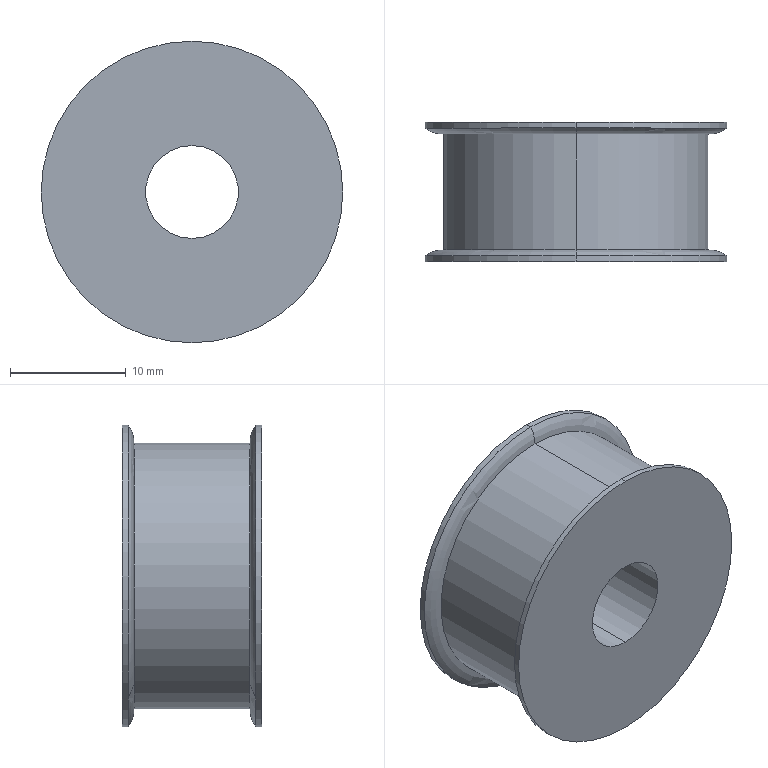Part | SolidWorks | features Revolution 2 | 1 solid | 14 faces | box 26 x 12 x 26 mm | volume 4546 mm3 | cylinder 8 | torus 4 | plane 2 | commonest cylinder face diameters 26 x4 8 x2 22.92 x2
STEP:
#1=CARTESIAN_POINT('',(0.,-5.5,-13.));
#2=VERTEX_POINT('',#1);
#3=CARTESIAN_POINT('',(0.,-5.5,13.));
#4=VERTEX_POINT('',#3);
#5=CARTESIAN_POINT('',(0.,-5.5,0.));
#6=DIRECTION('',(0.,-1.,0.));
#7=DIRECTION('',(0.,0.,-1.));
#8=AXIS2_PLACEMENT_3D('',#5,#6,#7);
#9=CIRCLE('',#8,13.);
#10=EDGE_CURVE('',#2,#4,#9,.T.);
#11=ORIENTED_EDGE('',*,*,#10,.T.);
#12=CARTESIAN_POINT('',(0.,-6.,13.));
#13=VERTEX_POINT('',#12);
#14=CARTESIAN_POINT('',(0.,0.,13.));
#15=DIRECTION('',(0.,-1.,0.));
#16=VECTOR('',#15,1000.);
#17=LINE('',#14,#16);
#18=EDGE_CURVE('',#4,#13,#17,.T.);
#19=ORIENTED_EDGE('',*,*,#18,.T.);
#20=CARTESIAN_POINT('',(0.,-6.,-13.));
#21=VERTEX_POINT('',#20);
#22=CARTESIAN_POINT('',(0.,-6.,0.));
#23=DIRECTION('',(0.,-1.,0.));
#24=DIRECTION('',(0.,0.,-1.));
#25=AXIS2_PLACEMENT_3D('',#22,#23,#24);
#26=CIRCLE('',#25,13.);
#27=EDGE_CURVE('',#21,#13,#26,.T.);
#28=ORIENTED_EDGE('',*,*,#27,.F.);
#29=CARTESIAN_POINT('',(0.,0.,-13.));
#30=DIRECTION('',(0.,-1.,0.));
#31=VECTOR('',#30,1000.);
#32=LINE('',#29,#31);
#33=EDGE_CURVE('',#2,#21,#32,.T.);
#34=ORIENTED_EDGE('',*,*,#33,.F.);
#35=EDGE_LOOP('',(#11,#19,#28,#34));
#36=FACE_OUTER_BOUND('',#35,.T.);
#37=CARTESIAN_POINT('',(0.,0.,0.));
#38=DIRECTION('',(0.,-1.,0.));
#39=DIRECTION('',(0.,0.,-1.));
#40=AXIS2_PLACEMENT_3D('',#37,#38,#39);
#41=CYLINDRICAL_SURFACE('',#40,13.);
#42=ADVANCED_FACE('',(#36),#41,.T.);
#43=CARTESIAN_POINT('',(0.,-5.,-11.46));
#44=VERTEX_POINT('',#43);
#45=CARTESIAN_POINT('',(0.,-5.,11.46));
#46=VERTEX_POINT('',#45);
#47=CARTESIAN_POINT('',(0.,-5.,0.));
#48=DIRECTION('',(0.,-1.,0.));
#49=DIRECTION('',(0.,0.,-1.));
#50=AXIS2_PLACEMENT_3D('',#47,#48,#49);
#51=CIRCLE('',#50,11.46);
#52=EDGE_CURVE('',#44,#46,#51,.T.);
#53=ORIENTED_EDGE('',*,*,#52,.T.);
#54=CARTESIAN_POINT('',(0.,-7.622,11.46));
#55=DIRECTION('',(1.,0.,0.));
#56=DIRECTION('',(0.,0.,-1.));
#57=AXIS2_PLACEMENT_3D('',#54,#55,#56);
#58=CIRCLE('',#57,2.622);
#59=EDGE_CURVE('',#46,#4,#58,.T.);
#60=ORIENTED_EDGE('',*,*,#59,.T.);
#61=ORIENTED_EDGE('',*,*,#10,.F.);
#62=CARTESIAN_POINT('',(0.,-7.622,-11.46));
#63=DIRECTION('',(-1.,0.,0.));
#64=DIRECTION('',(0.,0.,1.));
#65=AXIS2_PLACEMENT_3D('',#62,#63,#64);
#66=CIRCLE('',#65,2.622);
#67=EDGE_CURVE('',#44,#2,#66,.T.);
#68=ORIENTED_EDGE('',*,*,#67,.F.);
#69=EDGE_LOOP('',(#53,#60,#61,#68));
#70=FACE_OUTER_BOUND('',#69,.T.);
#71=CARTESIAN_POINT('',(0.,-7.622,0.));
#72=DIRECTION('',(0.,-1.,0.));
#73=DIRECTION('',(0.,0.,-1.));
#74=AXIS2_PLACEMENT_3D('',#71,#72,#73);
#75=TOROIDAL_SURFACE('',#74,11.46,2.622);
#76=ADVANCED_FACE('',(#70),#75,.T.);
#77=CARTESIAN_POINT('',(0.,6.,-13.));
#78=VERTEX_POINT('',#77);
#79=CARTESIAN_POINT('',(0.,6.,13.));
#80=VERTEX_POINT('',#79);
#81=CARTESIAN_POINT('',(0.,6.,0.));
#82=DIRECTION('',(0.,-1.,0.));
#83=DIRECTION('',(0.,0.,-1.));
#84=AXIS2_PLACEMENT_3D('',#81,#82,#83);
#85=CIRCLE('',#84,13.);
#86=EDGE_CURVE('',#78,#80,#85,.T.);
#87=ORIENTED_EDGE('',*,*,#86,.T.);
#88=CARTESIAN_POINT('',(0.,5.5,13.));
#89=VERTEX_POINT('',#88);
#90=CARTESIAN_POINT('',(0.,0.,13.));
#91=DIRECTION('',(0.,-1.,0.));
#92=VECTOR('',#91,1000.);
#93=LINE('',#90,#92);
#94=EDGE_CURVE('',#80,#89,#93,.T.);
#95=ORIENTED_EDGE('',*,*,#94,.T.);
#96=CARTESIAN_POINT('',(0.,5.5,-13.));
#97=VERTEX_POINT('',#96);
#98=CARTESIAN_POINT('',(0.,5.5,0.));
#99=DIRECTION('',(0.,-1.,0.));
#100=DIRECTION('',(0.,0.,-1.));
#101=AXIS2_PLACEMENT_3D('',#98,#99,#100);
#102=CIRCLE('',#101,13.);
#103=EDGE_CURVE('',#97,#89,#102,.T.);
#104=ORIENTED_EDGE('',*,*,#103,.F.);
#105=CARTESIAN_POINT('',(0.,0.,-13.));
#106=DIRECTION('',(0.,-1.,0.));
#107=VECTOR('',#106,1000.);
#108=LINE('',#105,#107);
#109=EDGE_CURVE('',#78,#97,#108,.T.);
#110=ORIENTED_EDGE('',*,*,#109,.F.);
#111=EDGE_LOOP('',(#87,#95,#104,#110));
#112=FACE_OUTER_BOUND('',#111,.T.);
#113=CARTESIAN_POINT('',(0.,0.,0.));
#114=DIRECTION('',(0.,-1.,0.));
#115=DIRECTION('',(0.,0.,-1.));
#116=AXIS2_PLACEMENT_3D('',#113,#114,#115);
#117=CYLINDRICAL_SURFACE('',#116,13.);
#118=ADVANCED_FACE('',(#112),#117,.T.);
#119=ORIENTED_EDGE('',*,*,#103,.T.);
#120=CARTESIAN_POINT('',(0.,5.,11.46));
#121=VERTEX_POINT('',#120);
#122=CARTESIAN_POINT('',(0.,7.622,11.46));
#123=DIRECTION('',(1.,0.,0.));
#124=DIRECTION('',(0.,0.,-1.));
#125=AXIS2_PLACEMENT_3D('',#122,#123,#124);
#126=CIRCLE('',#125,2.622);
#127=EDGE_CURVE('',#89,#121,#126,.T.);
#128=ORIENTED_EDGE('',*,*,#127,.T.);
#129=CARTESIAN_POINT('',(0.,5.,-11.46));
#130=VERTEX_POINT('',#129);
#131=CARTESIAN_POINT('',(0.,5.,0.));
#132=DIRECTION('',(0.,-1.,0.));
#133=DIRECTION('',(0.,0.,-1.));
#134=AXIS2_PLACEMENT_3D('',#131,#132,#133);
#135=CIRCLE('',#134,11.46);
#136=EDGE_CURVE('',#130,#121,#135,.T.);
#137=ORIENTED_EDGE('',*,*,#136,.F.);
#138=CARTESIAN_POINT('',(0.,7.622,-11.46));
#139=DIRECTION('',(-1.,0.,0.));
#140=DIRECTION('',(0.,0.,1.));
#141=AXIS2_PLACEMENT_3D('',#138,#139,#140);
#142=CIRCLE('',#141,2.622);
#143=EDGE_CURVE('',#97,#130,#142,.T.);
#144=ORIENTED_EDGE('',*,*,#143,.F.);
#145=EDGE_LOOP('',(#119,#128,#137,#144));
#146=FACE_OUTER_BOUND('',#145,.T.);
#147=CARTESIAN_POINT('',(0.,7.622,0.));
#148=DIRECTION('',(0.,-1.,0.));
#149=DIRECTION('',(0.,0.,-1.));
#150=AXIS2_PLACEMENT_3D('',#147,#148,#149);
#151=TOROIDAL_SURFACE('',#150,11.46,2.622);
#152=ADVANCED_FACE('',(#146),#151,.T.);
#153=CARTESIAN_POINT('',(0.,6.,4.));
#154=VERTEX_POINT('',#153);
#155=CARTESIAN_POINT('',(0.,6.,-4.));
#156=VERTEX_POINT('',#155);
#157=CARTESIAN_POINT('',(0.,6.,0.));
#158=DIRECTION('',(0.,-1.,0.));
#159=DIRECTION('',(0.,0.,-1.));
#160=AXIS2_PLACEMENT_3D('',#157,#158,#159);
#161=CIRCLE('',#160,4.);
#162=EDGE_CURVE('',#154,#156,#161,.T.);
#163=ORIENTED_EDGE('',*,*,#162,.F.);
#164=CARTESIAN_POINT('',(0.,-6.,4.));
#165=VERTEX_POINT('',#164);
#166=CARTESIAN_POINT('',(0.,0.,4.));
#167=DIRECTION('',(0.,-1.,0.));
#168=VECTOR('',#167,1000.);
#169=LINE('',#166,#168);
#170=EDGE_CURVE('',#154,#165,#169,.T.);
#171=ORIENTED_EDGE('',*,*,#170,.T.);
#172=CARTESIAN_POINT('',(0.,-6.,-4.));
#173=VERTEX_POINT('',#172);
#174=CARTESIAN_POINT('',(0.,-6.,0.));
#175=DIRECTION('',(0.,-1.,0.));
#176=DIRECTION('',(0.,0.,-1.));
#177=AXIS2_PLACEMENT_3D('',#174,#175,#176);
#178=CIRCLE('',#177,4.);
#179=EDGE_CURVE('',#165,#173,#178,.T.);
#180=ORIENTED_EDGE('',*,*,#179,.T.);
#181=CARTESIAN_POINT('',(0.,0.,-4.));
#182=DIRECTION('',(0.,-1.,0.));
#183=VECTOR('',#182,1000.);
#184=LINE('',#181,#183);
#185=EDGE_CURVE('',#156,#173,#184,.T.);
#186=ORIENTED_EDGE('',*,*,#185,.F.);
#187=EDGE_LOOP('',(#163,#171,#180,#186));
#188=FACE_OUTER_BOUND('',#187,.T.);
#189=CARTESIAN_POINT('',(0.,0.,0.));
#190=DIRECTION('',(0.,-1.,0.));
#191=DIRECTION('',(0.,0.,-1.));
#192=AXIS2_PLACEMENT_3D('',#189,#190,#191);
#193=CYLINDRICAL_SURFACE('',#192,4.);
#194=ADVANCED_FACE('',(#188),#193,.F.);
#195=ORIENTED_EDGE('',*,*,#136,.T.);
#196=CARTESIAN_POINT('',(0.,0.,11.46));
#197=DIRECTION('',(0.,-1.,0.));
#198=VECTOR('',#197,1000.);
#199=LINE('',#196,#198);
#200=EDGE_CURVE('',#121,#46,#199,.T.);
#201=ORIENTED_EDGE('',*,*,#200,.T.);
#202=ORIENTED_EDGE('',*,*,#52,.F.);
#203=CARTESIAN_POINT('',(0.,0.,-11.46));
#204=DIRECTION('',(0.,-1.,0.));
#205=VECTOR('',#204,1000.);
#206=LINE('',#203,#205);
#207=EDGE_CURVE('',#130,#44,#206,.T.);
#208=ORIENTED_EDGE('',*,*,#207,.F.);
#209=EDGE_LOOP('',(#195,#201,#202,#208));
#210=FACE_OUTER_BOUND('',#209,.T.);
#211=CARTESIAN_POINT('',(0.,0.,0.));
#212=DIRECTION('',(0.,-1.,0.));
#213=DIRECTION('',(0.,0.,-1.));
#214=AXIS2_PLACEMENT_3D('',#211,#212,#213);
#215=CYLINDRICAL_SURFACE('',#214,11.46);
#216=ADVANCED_FACE('',(#210),#215,.T.);
#217=ORIENTED_EDGE('',*,*,#200,.F.);
#218=CARTESIAN_POINT('',(0.,5.,0.));
#219=DIRECTION('',(0.,-1.,0.));
#220=DIRECTION('',(0.,0.,-1.));
#221=AXIS2_PLACEMENT_3D('',#218,#219,#220);
#222=CIRCLE('',#221,11.46);
#223=EDGE_CURVE('',#121,#130,#222,.T.);
#224=ORIENTED_EDGE('',*,*,#223,.T.);
#225=ORIENTED_EDGE('',*,*,#207,.T.);
#226=CARTESIAN_POINT('',(0.,-5.,0.));
#227=DIRECTION('',(0.,-1.,0.));
#228=DIRECTION('',(0.,0.,-1.));
#229=AXIS2_PLACEMENT_3D('',#226,#227,#228);
#230=CIRCLE('',#229,11.46);
#231=EDGE_CURVE('',#46,#44,#230,.T.);
#232=ORIENTED_EDGE('',*,*,#231,.F.);
#233=EDGE_LOOP('',(#217,#224,#225,#232));
#234=FACE_OUTER_BOUND('',#233,.T.);
#235=CARTESIAN_POINT('',(0.,0.,0.));
#236=DIRECTION('',(0.,-1.,0.));
#237=DIRECTION('',(0.,0.,-1.));
#238=AXIS2_PLACEMENT_3D('',#235,#236,#237);
#239=CYLINDRICAL_SURFACE('',#238,11.46);
#240=ADVANCED_FACE('',(#234),#239,.T.);
#241=CARTESIAN_POINT('',(0.,-6.,0.));
#242=DIRECTION('',(0.,-1.,0.));
#243=DIRECTION('',(0.,0.,-1.));
#244=AXIS2_PLACEMENT_3D('',#241,#242,#243);
#245=CIRCLE('',#244,4.);
#246=EDGE_CURVE('',#173,#165,#245,.T.);
#247=ORIENTED_EDGE('',*,*,#246,.F.);
#248=ORIENTED_EDGE('',*,*,#179,.F.);
#249=EDGE_LOOP('',(#247,#248));
#250=FACE_BOUND('',#249,.T.);
#251=ORIENTED_EDGE('',*,*,#27,.T.);
#252=CARTESIAN_POINT('',(0.,-6.,0.));
#253=DIRECTION('',(0.,-1.,0.));
#254=DIRECTION('',(0.,0.,-1.));
#255=AXIS2_PLACEMENT_3D('',#252,#253,#254);
#256=CIRCLE('',#255,13.);
#257=EDGE_CURVE('',#13,#21,#256,.T.);
#258=ORIENTED_EDGE('',*,*,#257,.T.);
#259=EDGE_LOOP('',(#251,#258));
#260=FACE_OUTER_BOUND('',#259,.T.);
#261=CARTESIAN_POINT('',(8.,-6.,0.));
#262=DIRECTION('',(0.,-1.,0.));
#263=DIRECTION('',(0.,0.,-1.));
#264=AXIS2_PLACEMENT_3D('',#261,#262,#263);
#265=PLANE('',#264);
#266=ADVANCED_FACE('',(#250,#260),#265,.T.);
#267=ORIENTED_EDGE('',*,*,#170,.F.);
#268=CARTESIAN_POINT('',(0.,6.,0.));
#269=DIRECTION('',(0.,-1.,0.));
#270=DIRECTION('',(0.,0.,-1.));
#271=AXIS2_PLACEMENT_3D('',#268,#269,#270);
#272=CIRCLE('',#271,4.);
#273=EDGE_CURVE('',#156,#154,#272,.T.);
#274=ORIENTED_EDGE('',*,*,#273,.F.);
#275=ORIENTED_EDGE('',*,*,#185,.T.);
#276=ORIENTED_EDGE('',*,*,#246,.T.);
#277=EDGE_LOOP('',(#267,#274,#275,#276));
#278=FACE_OUTER_BOUND('',#277,.T.);
#279=CARTESIAN_POINT('',(0.,0.,0.));
#280=DIRECTION('',(0.,-1.,0.));
#281=DIRECTION('',(0.,0.,-1.));
#282=AXIS2_PLACEMENT_3D('',#279,#280,#281);
#283=CYLINDRICAL_SURFACE('',#282,4.);
#284=ADVANCED_FACE('',(#278),#283,.F.);
#285=ORIENTED_EDGE('',*,*,#273,.T.);
#286=ORIENTED_EDGE('',*,*,#162,.T.);
#287=EDGE_LOOP('',(#285,#286));
#288=FACE_BOUND('',#287,.T.);
#289=ORIENTED_EDGE('',*,*,#86,.F.);
#290=CARTESIAN_POINT('',(0.,6.,0.));
#291=DIRECTION('',(0.,-1.,0.));
#292=DIRECTION('',(0.,0.,-1.));
#293=AXIS2_PLACEMENT_3D('',#290,#291,#292);
#294=CIRCLE('',#293,13.);
#295=EDGE_CURVE('',#80,#78,#294,.T.);
#296=ORIENTED_EDGE('',*,*,#295,.F.);
#297=EDGE_LOOP('',(#289,#296));
#298=FACE_OUTER_BOUND('',#297,.T.);
#299=CARTESIAN_POINT('',(8.,6.,0.));
#300=DIRECTION('',(0.,1.,0.));
#301=DIRECTION('',(0.,0.,1.));
#302=AXIS2_PLACEMENT_3D('',#299,#300,#301);
#303=PLANE('',#302);
#304=ADVANCED_FACE('',(#288,#298),#303,.T.);
#305=ORIENTED_EDGE('',*,*,#127,.F.);
#306=CARTESIAN_POINT('',(0.,5.5,0.));
#307=DIRECTION('',(0.,-1.,0.));
#308=DIRECTION('',(0.,0.,-1.));
#309=AXIS2_PLACEMENT_3D('',#306,#307,#308);
#310=CIRCLE('',#309,13.);
#311=EDGE_CURVE('',#89,#97,#310,.T.);
#312=ORIENTED_EDGE('',*,*,#311,.T.);
#313=ORIENTED_EDGE('',*,*,#143,.T.);
#314=ORIENTED_EDGE('',*,*,#223,.F.);
#315=EDGE_LOOP('',(#305,#312,#313,#314));
#316=FACE_OUTER_BOUND('',#315,.T.);
#317=CARTESIAN_POINT('',(0.,7.622,0.));
#318=DIRECTION('',(0.,-1.,0.));
#319=DIRECTION('',(0.,0.,-1.));
#320=AXIS2_PLACEMENT_3D('',#317,#318,#319);
#321=TOROIDAL_SURFACE('',#320,11.46,2.622);
#322=ADVANCED_FACE('',(#316),#321,.T.);
#323=ORIENTED_EDGE('',*,*,#94,.F.);
#324=ORIENTED_EDGE('',*,*,#295,.T.);
#325=ORIENTED_EDGE('',*,*,#109,.T.);
#326=ORIENTED_EDGE('',*,*,#311,.F.);
#327=EDGE_LOOP('',(#323,#324,#325,#326));
#328=FACE_OUTER_BOUND('',#327,.T.);
#329=CARTESIAN_POINT('',(0.,0.,0.));
#330=DIRECTION('',(0.,-1.,0.));
#331=DIRECTION('',(0.,0.,-1.));
#332=AXIS2_PLACEMENT_3D('',#329,#330,#331);
#333=CYLINDRICAL_SURFACE('',#332,13.);
#334=ADVANCED_FACE('',(#328),#333,.T.);
#335=ORIENTED_EDGE('',*,*,#59,.F.);
#336=ORIENTED_EDGE('',*,*,#231,.T.);
#337=ORIENTED_EDGE('',*,*,#67,.T.);
#338=CARTESIAN_POINT('',(0.,-5.5,0.));
#339=DIRECTION('',(0.,-1.,0.));
#340=DIRECTION('',(0.,0.,-1.));
#341=AXIS2_PLACEMENT_3D('',#338,#339,#340);
#342=CIRCLE('',#341,13.);
#343=EDGE_CURVE('',#4,#2,#342,.T.);
#344=ORIENTED_EDGE('',*,*,#343,.F.);
#345=EDGE_LOOP('',(#335,#336,#337,#344));
#346=FACE_OUTER_BOUND('',#345,.T.);
#347=CARTESIAN_POINT('',(0.,-7.622,0.));
#348=DIRECTION('',(0.,-1.,0.));
#349=DIRECTION('',(0.,0.,-1.));
#350=AXIS2_PLACEMENT_3D('',#347,#348,#349);
#351=TOROIDAL_SURFACE('',#350,11.46,2.622);
#352=ADVANCED_FACE('',(#346),#351,.T.);
#353=ORIENTED_EDGE('',*,*,#18,.F.);
#354=ORIENTED_EDGE('',*,*,#343,.T.);
#355=ORIENTED_EDGE('',*,*,#33,.T.);
#356=ORIENTED_EDGE('',*,*,#257,.F.);
#357=EDGE_LOOP('',(#353,#354,#355,#356));
#358=FACE_OUTER_BOUND('',#357,.T.);
#359=CARTESIAN_POINT('',(0.,0.,0.));
#360=DIRECTION('',(0.,-1.,0.));
#361=DIRECTION('',(0.,0.,-1.));
#362=AXIS2_PLACEMENT_3D('',#359,#360,#361);
#363=CYLINDRICAL_SURFACE('',#362,13.);
#364=ADVANCED_FACE('',(#358),#363,.T.);
#365=CLOSED_SHELL('',(#42,#76,#118,#152,#194,#216,#240,#266,#284,#304,#322,#334,#352,#364));
#366=MANIFOLD_SOLID_BREP('',#365);
#367=CARTESIAN_POINT('',(0.,0.,0.));
#368=DIRECTION('',(0.,0.,1.));
#369=DIRECTION('',(1.,0.,0.));
#370=AXIS2_PLACEMENT_3D('',#367,#368,#369);
#371=(LENGTH_UNIT()NAMED_UNIT(*)SI_UNIT(.MILLI.,.METRE.));
#372=UNCERTAINTY_MEASURE_WITH_UNIT(LENGTH_MEASURE(0.00001),#371,'','');
#373=(NAMED_UNIT(*)PLANE_ANGLE_UNIT()SI_UNIT($,.RADIAN.));
#374=(NAMED_UNIT(*)SI_UNIT($,.STERADIAN.)SOLID_ANGLE_UNIT());
#375=(GEOMETRIC_REPRESENTATION_CONTEXT(3)GLOBAL_UNCERTAINTY_ASSIGNED_CONTEXT((#372))GLOBAL_UNIT_ASSIGNED_CONTEXT((#371,#373,#374))REPRESENTATION_CONTEXT('',''));
#376=ADVANCED_BREP_SHAPE_REPRESENTATION('',(#366,#370),#375);